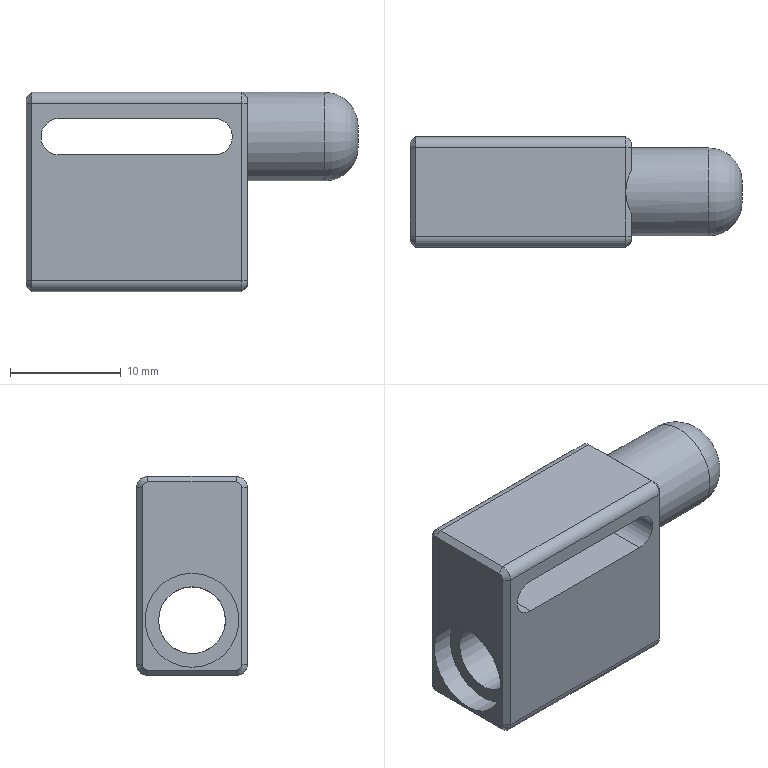CAM job | NX | 3+2 milling, drilling | part box 30 x 10 x 18 mm | stock box 35 x 12 x 23 mm
Tools:
number,name,description,diameter,corner_radius,flute_length,length,flutes
4,D4,平底铣刀-粗,4.0,0.0,25.0,75.0,2
9,D10,平底铣刀-粗,10.0,0.0,35.0,75.0,2
18,D4-J,平底铣刀-精,4.0,0.0,50.0,75.0,2
7,D6-J,平底铣刀-精,6.0,0.0,25.0,75.0,2
10,D10-J,平底铣刀-精,10.0,0.0,35.0,75.0,2
19,D6R0.5,圆鼻刀-粗,6.0,0.5,50.0,75.0,2
1,D80R0.8飞刀,圆鼻刀-粗,80.0,0.8,50.0,75.0,2
2,D6倒角刀,倒角刀,6.0,0.0,3.0,25.0,2
17,ZT5.9,Drilling Tool,5.9,0.0,35.0,50.0,2
Operations:
program,operation,operation_type,tool,method,geometry_group,spindle_rpm,surface_speed,feed_per_tooth,feed_cut,feed_plunge,cut_length_mm,path_length_mm,cut_time_min,machine_time_min
B,面铣自动飞面开粗_COPY,FaceMilling,D10,分层开粗-切深K-步距G,W-B,8000.0,251.327,0.1875,3000.0,100.0,808.661,921.616,0.2696,0.2808
B,型腔铣开粗-中_COPY,CavityMilling,D10,分层开粗-切深K-步距G,W-B,8000.0,251.32,0.25,4000.0,100.0,4978.337,5837.199,1.245,1.378
B,面铣自动飞面精光_COPY,FaceMilling,D6-J,侧刃精光-切深K-步距G,W-B,7000.0,219.911,0.0714,1000.0,100.0,108.0,144.0,0.108,0.1116
B,等高螺旋爬面_COPY,ZLevelMilling,D6R0.5,等高爬面-切深K-步距G,W-B,7000.0,131.947,0.2857,4000.0,100.0,2041.368,2081.868,0.5103,0.5144
B,铣倒角_2,PlanarMilling,D6倒角刀,METHOD,W-B,7000.0,131.947,0.0429,600.0,100.0,10,73.4,0.0167,0.023
B,底壁铣精光底面-中_COPY,VolumeBased25DMillingOperation,D6-J,精光步距切深关,W-B,7000.0,175.0,0.0536,1500.0,100.0,52.44,99.04,0.035,0.0396
B,等高精光-中_COPY,ZLevelMilling,D6-J,侧刃精光-切深K-步距G,W-B,8000.0,150.792,0.0625,1000.0,100.0,49.107,86.707,0.0491,0.0529
B,等高精光往复爬面_COPY,ZLevelMilling,D6-J,等高爬面-切深K-步距G,W-B,7000.0,131.947,0.2857,4000.0,100.0,3094.565,3144.175,0.7736,0.7786
A,顶面,FaceMilling,D80R0.8飞刀,侧刃精光-切深K-步距G,W-A,5000.0,1256.637,0.1,1000.0,100.0,112.0,148.0,0.112,0.1156
A,外形粗_2,VolumeBased25DMillingOperation,D10,METHOD,W-A,8000.0,251.327,0.3125,5000.0,80.0,2418.767,2478.267,0.4838,0.4897
A,沉头孔打点-深0.8,Operation,D6倒角刀,NONE,W-A,8000.0,150.796,0.0312,500.0,90.0,1.8,43.6,0.0036,0.0078
A,沉头孔-钻孔0段,Operation,ZT5.9,NONE,W-A,2800.0,53.219,0.0357,200.0,90.0,24.703,89.406,0.1235,0.13
A,铣孔开粗D4_1,CylinderMilling,D4,NONE,W-A,8000.0,100.531,0.075,1200.0,100.0,132.865,174.365,0.1107,0.1149
A,铣倒角_1,PlanarMilling,D6倒角刀,NONE,W-A,8000.0,150.796,0.0312,500.0,100.0,35.539,71.539,0.0711,0.0747
A,底壁铣倒角_COPY,VolumeBased25DMillingOperation,D6倒角刀,爬面_倒角-切深0-步距G,W-A,6500.0,122.519,0.1154,1500.0,100.0,65.601,105.001,0.0437,0.0477
A,底壁铣精光侧面-中-选底面_COPY,VolumeBased25DMillingOperation,D4-J,侧刃精光-切深K-步距G,W-A,6000.0,75.398,0.05,600.0,100.0,20.02,42.42,0.0334,0.0356
A,底壁铣精光侧面-中_COPY,VolumeBased25DMillingOperation,D4-J,侧刃精光-切深K-步距G,W-A,6000.0,75.398,0.0417,500.0,100.0,49.71,107.916,0.0994,0.1052
A,外形半精_2,VolumeBased25DMillingOperation,D10-J,METHOD,W-A,8000.0,251.327,0.0625,1000.0,100.0,181.338,324.851,0.1813,0.1957